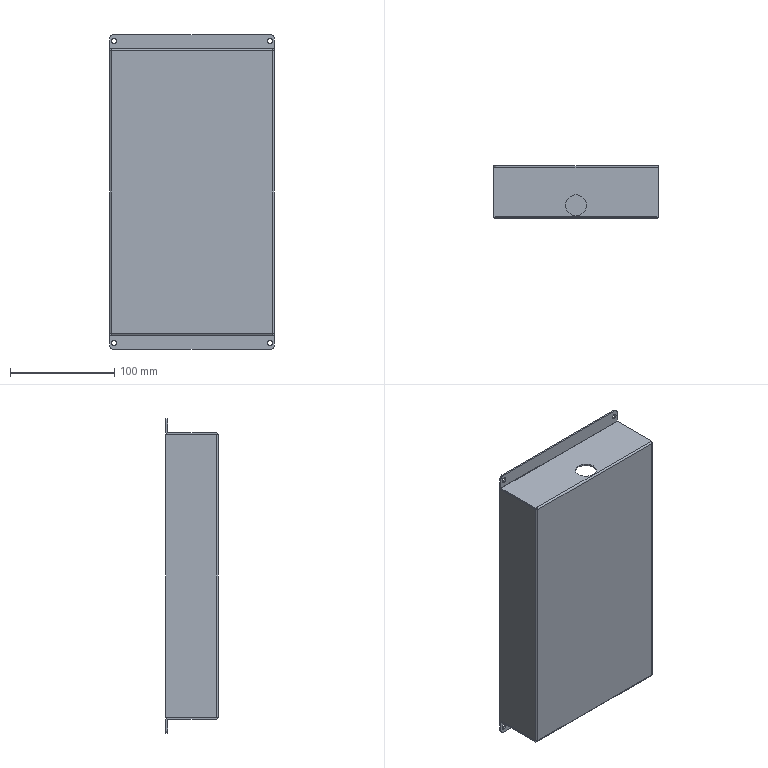Part | STEP file | HESS-408-70-15W-W-33-front door electrical control box | 1 solid | 60 faces | box 158 x 50 x 302 mm | volume 132853 mm3 | plane 34 | cylinder 26 | commonest cylinder face diameters 5 x8 0.2 x6 3.2 x6 6 x4 20 x2